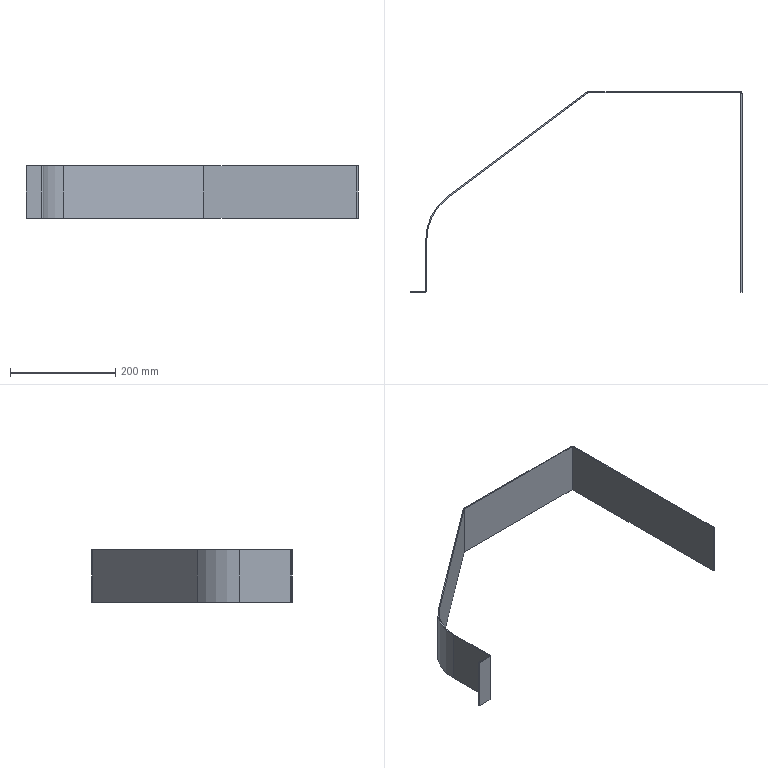Part | SolidWorks | features ICE 5, DeleteBody 4, Split 4, Extrusion 1, FlatPattern 1, SheetMetal 1, Shell 1, SolidToSheetMetal 1 | 1 solid | 38 faces | box 630 x 380 x 100 mm | volume 244808 mm3 | plane 30 | cylinder 8 | commonest cylinder face diameters 2 x3 6 x3 196 x1 200 x1
STEP:
#1=CARTESIAN_POINT('',(-1098.,3.,-198.));
#2=VERTEX_POINT('',#1);
#3=CARTESIAN_POINT('',(-1100.,3.,-198.));
#4=VERTEX_POINT('',#3);
#5=CARTESIAN_POINT('',(-1100.,3.,-198.));
#6=DIRECTION('',(-1.,0.,0.));
#7=VECTOR('',#6,1000.);
#8=LINE('',#5,#7);
#9=EDGE_CURVE('',#2,#4,#8,.T.);
#10=ORIENTED_EDGE('',*,*,#9,.F.);
#11=CARTESIAN_POINT('',(-1098.,100.,-198.));
#12=VERTEX_POINT('',#11);
#13=CARTESIAN_POINT('',(-1098.,100.,-198.));
#14=DIRECTION('',(0.,1.,0.));
#15=VECTOR('',#14,1000.);
#16=LINE('',#13,#15);
#17=EDGE_CURVE('',#2,#12,#16,.T.);
#18=ORIENTED_EDGE('',*,*,#17,.T.);
#19=CARTESIAN_POINT('',(-1100.,100.,-198.));
#20=VERTEX_POINT('',#19);
#21=CARTESIAN_POINT('',(-1100.,100.,-198.));
#22=DIRECTION('',(-1.,0.,0.));
#23=VECTOR('',#22,1000.);
#24=LINE('',#21,#23);
#25=EDGE_CURVE('',#12,#20,#24,.T.);
#26=ORIENTED_EDGE('',*,*,#25,.T.);
#27=CARTESIAN_POINT('',(-1100.,100.,-198.));
#28=DIRECTION('',(0.,1.,0.));
#29=VECTOR('',#28,1000.);
#30=LINE('',#27,#29);
#31=EDGE_CURVE('',#4,#20,#30,.T.);
#32=ORIENTED_EDGE('',*,*,#31,.F.);
#33=EDGE_LOOP('',(#10,#18,#26,#32));
#34=FACE_OUTER_BOUND('',#33,.T.);
#35=CARTESIAN_POINT('',(-1100.,100.,-198.));
#36=DIRECTION('',(0.,0.,1.));
#37=DIRECTION('',(0.,1.,0.));
#38=AXIS2_PLACEMENT_3D('',#35,#36,#37);
#39=PLANE('',#38);
#40=ADVANCED_FACE('',(#34),#39,.T.);
#41=ORIENTED_EDGE('',*,*,#25,.F.);
#42=CARTESIAN_POINT('',(-1058.8,178.4,-198.));
#43=VERTEX_POINT('',#42);
#44=CARTESIAN_POINT('',(-1000.,100.,-198.));
#45=DIRECTION('',(0.,0.,-1.));
#46=DIRECTION('',(1.,0.,0.));
#47=AXIS2_PLACEMENT_3D('',#44,#45,#46);
#48=CIRCLE('',#47,98.);
#49=EDGE_CURVE('',#12,#43,#48,.T.);
#50=ORIENTED_EDGE('',*,*,#49,.T.);
#51=CARTESIAN_POINT('',(-1060.,180.,-198.));
#52=VERTEX_POINT('',#51);
#53=CARTESIAN_POINT('',(-1060.,180.,-198.));
#54=DIRECTION('',(-0.6,0.8,0.));
#55=VECTOR('',#54,1000.);
#56=LINE('',#53,#55);
#57=EDGE_CURVE('',#43,#52,#56,.T.);
#58=ORIENTED_EDGE('',*,*,#57,.T.);
#59=CARTESIAN_POINT('',(-1000.,100.,-198.));
#60=DIRECTION('',(0.,0.,-1.));
#61=DIRECTION('',(1.,0.,0.));
#62=AXIS2_PLACEMENT_3D('',#59,#60,#61);
#63=CIRCLE('',#62,100.);
#64=EDGE_CURVE('',#20,#52,#63,.T.);
#65=ORIENTED_EDGE('',*,*,#64,.F.);
#66=EDGE_LOOP('',(#41,#50,#58,#65));
#67=FACE_OUTER_BOUND('',#66,.T.);
#68=CARTESIAN_POINT('',(-1000.,100.,-198.));
#69=DIRECTION('',(0.,0.,-1.));
#70=DIRECTION('',(-1.,0.,0.));
#71=AXIS2_PLACEMENT_3D('',#68,#69,#70);
#72=PLANE('',#71);
#73=ADVANCED_FACE('',(#67),#72,.F.);
#74=ORIENTED_EDGE('',*,*,#57,.F.);
#75=CARTESIAN_POINT('',(-792.933,377.8,-198.));
#76=VERTEX_POINT('',#75);
#77=CARTESIAN_POINT('',(-1058.8,178.4,-198.));
#78=DIRECTION('',(0.8,0.6,0.));
#79=VECTOR('',#78,1000.);
#80=LINE('',#77,#79);
#81=EDGE_CURVE('',#43,#76,#80,.T.);
#82=ORIENTED_EDGE('',*,*,#81,.T.);
#83=CARTESIAN_POINT('',(-794.133,379.4,-198.));
#84=VERTEX_POINT('',#83);
#85=CARTESIAN_POINT('',(-794.133,379.4,-198.));
#86=DIRECTION('',(-0.6,0.8,0.));
#87=VECTOR('',#86,1000.);
#88=LINE('',#85,#87);
#89=EDGE_CURVE('',#76,#84,#88,.T.);
#90=ORIENTED_EDGE('',*,*,#89,.T.);
#91=CARTESIAN_POINT('',(-1060.,180.,-198.));
#92=DIRECTION('',(0.8,0.6,0.));
#93=VECTOR('',#92,1000.);
#94=LINE('',#91,#93);
#95=EDGE_CURVE('',#52,#84,#94,.T.);
#96=ORIENTED_EDGE('',*,*,#95,.F.);
#97=EDGE_LOOP('',(#74,#82,#90,#96));
#98=FACE_OUTER_BOUND('',#97,.T.);
#99=CARTESIAN_POINT('',(-1060.,180.,-198.));
#100=DIRECTION('',(0.,0.,1.));
#101=DIRECTION('',(0.8,0.6,0.));
#102=AXIS2_PLACEMENT_3D('',#99,#100,#101);
#103=PLANE('',#102);
#104=ADVANCED_FACE('',(#98),#103,.T.);
#105=ORIENTED_EDGE('',*,*,#89,.F.);
#106=CARTESIAN_POINT('',(-792.333,378.,-198.));
#107=VERTEX_POINT('',#106);
#108=CARTESIAN_POINT('',(-792.333,377.,-198.));
#109=DIRECTION('',(0.,0.,-1.));
#110=DIRECTION('',(1.,0.,0.));
#111=AXIS2_PLACEMENT_3D('',#108,#109,#110);
#112=CIRCLE('',#111,1.);
#113=EDGE_CURVE('',#76,#107,#112,.T.);
#114=ORIENTED_EDGE('',*,*,#113,.T.);
#115=CARTESIAN_POINT('',(-792.333,380.,-198.));
#116=VERTEX_POINT('',#115);
#117=CARTESIAN_POINT('',(-792.333,380.,-198.));
#118=DIRECTION('',(0.,1.,0.));
#119=VECTOR('',#118,1000.);
#120=LINE('',#117,#119);
#121=EDGE_CURVE('',#107,#116,#120,.T.);
#122=ORIENTED_EDGE('',*,*,#121,.T.);
#123=CARTESIAN_POINT('',(-792.333,377.,-198.));
#124=DIRECTION('',(0.,0.,-1.));
#125=DIRECTION('',(-1.,0.,0.));
#126=AXIS2_PLACEMENT_3D('',#123,#124,#125);
#127=CIRCLE('',#126,3.);
#128=EDGE_CURVE('',#84,#116,#127,.T.);
#129=ORIENTED_EDGE('',*,*,#128,.F.);
#130=EDGE_LOOP('',(#105,#114,#122,#129));
#131=FACE_OUTER_BOUND('',#130,.T.);
#132=CARTESIAN_POINT('',(-792.333,377.,-198.));
#133=DIRECTION('',(0.,0.,1.));
#134=DIRECTION('',(1.,0.,0.));
#135=AXIS2_PLACEMENT_3D('',#132,#133,#134);
#136=PLANE('',#135);
#137=ADVANCED_FACE('',(#131),#136,.T.);
#138=ORIENTED_EDGE('',*,*,#121,.F.);
#139=CARTESIAN_POINT('',(-503.,378.,-198.));
#140=VERTEX_POINT('',#139);
#141=CARTESIAN_POINT('',(-500.,378.,-198.));
#142=DIRECTION('',(-1.,0.,0.));
#143=VECTOR('',#142,1000.);
#144=LINE('',#141,#143);
#145=EDGE_CURVE('',#140,#107,#144,.T.);
#146=ORIENTED_EDGE('',*,*,#145,.F.);
#147=CARTESIAN_POINT('',(-503.,380.,-198.));
#148=VERTEX_POINT('',#147);
#149=CARTESIAN_POINT('',(-503.,380.,-198.));
#150=DIRECTION('',(0.,1.,0.));
#151=VECTOR('',#150,1000.);
#152=LINE('',#149,#151);
#153=EDGE_CURVE('',#140,#148,#152,.T.);
#154=ORIENTED_EDGE('',*,*,#153,.T.);
#155=CARTESIAN_POINT('',(-2.,380.,-198.));
#156=DIRECTION('',(-1.,0.,0.));
#157=VECTOR('',#156,1000.);
#158=LINE('',#155,#157);
#159=EDGE_CURVE('',#148,#116,#158,.T.);
#160=ORIENTED_EDGE('',*,*,#159,.T.);
#161=EDGE_LOOP('',(#138,#146,#154,#160));
#162=FACE_OUTER_BOUND('',#161,.T.);
#163=CARTESIAN_POINT('',(-2.,380.,-198.));
#164=DIRECTION('',(0.,0.,-1.));
#165=DIRECTION('',(-1.,0.,0.));
#166=AXIS2_PLACEMENT_3D('',#163,#164,#165);
#167=PLANE('',#166);
#168=ADVANCED_FACE('',(#162),#167,.F.);
#169=ORIENTED_EDGE('',*,*,#153,.F.);
#170=CARTESIAN_POINT('',(-502.,377.,-198.));
#171=VERTEX_POINT('',#170);
#172=CARTESIAN_POINT('',(-503.,377.,-198.));
#173=DIRECTION('',(0.,0.,-1.));
#174=DIRECTION('',(1.,0.,0.));
#175=AXIS2_PLACEMENT_3D('',#172,#173,#174);
#176=CIRCLE('',#175,1.);
#177=EDGE_CURVE('',#140,#171,#176,.T.);
#178=ORIENTED_EDGE('',*,*,#177,.T.);
#179=CARTESIAN_POINT('',(-500.,377.,-198.));
#180=VERTEX_POINT('',#179);
#181=CARTESIAN_POINT('',(-500.,377.,-198.));
#182=DIRECTION('',(1.,0.,0.));
#183=VECTOR('',#182,1000.);
#184=LINE('',#181,#183);
#185=EDGE_CURVE('',#171,#180,#184,.T.);
#186=ORIENTED_EDGE('',*,*,#185,.T.);
#187=CARTESIAN_POINT('',(-503.,377.,-198.));
#188=DIRECTION('',(0.,0.,-1.));
#189=DIRECTION('',(1.,0.,0.));
#190=AXIS2_PLACEMENT_3D('',#187,#188,#189);
#191=CIRCLE('',#190,3.);
#192=EDGE_CURVE('',#148,#180,#191,.T.);
#193=ORIENTED_EDGE('',*,*,#192,.F.);
#194=EDGE_LOOP('',(#169,#178,#186,#193));
#195=FACE_OUTER_BOUND('',#194,.T.);
#196=CARTESIAN_POINT('',(-503.,377.,-198.));
#197=DIRECTION('',(0.,0.,-1.));
#198=DIRECTION('',(-1.,0.,0.));
#199=AXIS2_PLACEMENT_3D('',#196,#197,#198);
#200=PLANE('',#199);
#201=ADVANCED_FACE('',(#195),#200,.F.);
#202=ORIENTED_EDGE('',*,*,#185,.F.);
#203=CARTESIAN_POINT('',(-502.,0.,-198.));
#204=VERTEX_POINT('',#203);
#205=CARTESIAN_POINT('',(-502.,2.,-198.));
#206=DIRECTION('',(0.,1.,0.));
#207=VECTOR('',#206,1000.);
#208=LINE('',#205,#207);
#209=EDGE_CURVE('',#204,#171,#208,.T.);
#210=ORIENTED_EDGE('',*,*,#209,.F.);
#211=CARTESIAN_POINT('',(-500.,0.,-198.));
#212=VERTEX_POINT('',#211);
#213=CARTESIAN_POINT('',(-500.,0.,-198.));
#214=DIRECTION('',(1.,0.,0.));
#215=VECTOR('',#214,1000.);
#216=LINE('',#213,#215);
#217=EDGE_CURVE('',#204,#212,#216,.T.);
#218=ORIENTED_EDGE('',*,*,#217,.T.);
#219=CARTESIAN_POINT('',(-500.,375.,-198.));
#220=DIRECTION('',(0.,1.,0.));
#221=VECTOR('',#220,1000.);
#222=LINE('',#219,#221);
#223=EDGE_CURVE('',#212,#180,#222,.T.);
#224=ORIENTED_EDGE('',*,*,#223,.T.);
#225=EDGE_LOOP('',(#202,#210,#218,#224));
#226=FACE_OUTER_BOUND('',#225,.T.);
#227=CARTESIAN_POINT('',(-500.,375.,-198.));
#228=DIRECTION('',(0.,0.,-1.));
#229=DIRECTION('',(0.,1.,0.));
#230=AXIS2_PLACEMENT_3D('',#227,#228,#229);
#231=PLANE('',#230);
#232=ADVANCED_FACE('',(#226),#231,.F.);
#233=ORIENTED_EDGE('',*,*,#217,.F.);
#234=CARTESIAN_POINT('',(-502.,0.,-298.));
#235=VERTEX_POINT('',#234);
#236=CARTESIAN_POINT('',(-502.,0.,-200.));
#237=DIRECTION('',(0.,0.,1.));
#238=VECTOR('',#237,1000.);
#239=LINE('',#236,#238);
#240=EDGE_CURVE('',#235,#204,#239,.T.);
#241=ORIENTED_EDGE('',*,*,#240,.F.);
#242=CARTESIAN_POINT('',(-500.,0.,-298.));
#243=VERTEX_POINT('',#242);
#244=CARTESIAN_POINT('',(-500.,0.,-298.));
#245=DIRECTION('',(1.,0.,0.));
#246=VECTOR('',#245,1000.);
#247=LINE('',#244,#246);
#248=EDGE_CURVE('',#235,#243,#247,.T.);
#249=ORIENTED_EDGE('',*,*,#248,.T.);
#250=CARTESIAN_POINT('',(-500.,0.,-200.));
#251=DIRECTION('',(0.,0.,1.));
#252=VECTOR('',#251,1000.);
#253=LINE('',#250,#252);
#254=EDGE_CURVE('',#243,#212,#253,.T.);
#255=ORIENTED_EDGE('',*,*,#254,.T.);
#256=EDGE_LOOP('',(#233,#241,#249,#255));
#257=FACE_OUTER_BOUND('',#256,.T.);
#258=CARTESIAN_POINT('',(-500.,0.,-200.));
#259=DIRECTION('',(0.,1.,0.));
#260=DIRECTION('',(0.,0.,1.));
#261=AXIS2_PLACEMENT_3D('',#258,#259,#260);
#262=PLANE('',#261);
#263=ADVANCED_FACE('',(#257),#262,.F.);
#264=ORIENTED_EDGE('',*,*,#248,.F.);
#265=CARTESIAN_POINT('',(-502.,377.,-298.));
#266=VERTEX_POINT('',#265);
#267=CARTESIAN_POINT('',(-502.,2.,-298.));
#268=DIRECTION('',(0.,-1.,0.));
#269=VECTOR('',#268,1000.);
#270=LINE('',#267,#269);
#271=EDGE_CURVE('',#266,#235,#270,.T.);
#272=ORIENTED_EDGE('',*,*,#271,.F.);
#273=CARTESIAN_POINT('',(-500.,377.,-298.));
#274=VERTEX_POINT('',#273);
#275=CARTESIAN_POINT('',(-500.,377.,-298.));
#276=DIRECTION('',(1.,0.,0.));
#277=VECTOR('',#276,1000.);
#278=LINE('',#275,#277);
#279=EDGE_CURVE('',#266,#274,#278,.T.);
#280=ORIENTED_EDGE('',*,*,#279,.T.);
#281=CARTESIAN_POINT('',(-500.,2.,-298.));
#282=DIRECTION('',(0.,-1.,0.));
#283=VECTOR('',#282,1000.);
#284=LINE('',#281,#283);
#285=EDGE_CURVE('',#274,#243,#284,.T.);
#286=ORIENTED_EDGE('',*,*,#285,.T.);
#287=EDGE_LOOP('',(#264,#272,#280,#286));
#288=FACE_OUTER_BOUND('',#287,.T.);
#289=CARTESIAN_POINT('',(-500.,2.,-298.));
#290=DIRECTION('',(0.,0.,1.));
#291=DIRECTION('',(0.,-1.,0.));
#292=AXIS2_PLACEMENT_3D('',#289,#290,#291);
#293=PLANE('',#292);
#294=ADVANCED_FACE('',(#288),#293,.F.);
#295=ORIENTED_EDGE('',*,*,#279,.F.);
#296=CARTESIAN_POINT('',(-503.,378.,-298.));
#297=VERTEX_POINT('',#296);
#298=CARTESIAN_POINT('',(-503.,377.,-298.));
#299=DIRECTION('',(0.,0.,1.));
#300=DIRECTION('',(1.,0.,0.));
#301=AXIS2_PLACEMENT_3D('',#298,#299,#300);
#302=CIRCLE('',#301,1.);
#303=EDGE_CURVE('',#266,#297,#302,.T.);
#304=ORIENTED_EDGE('',*,*,#303,.T.);
#305=CARTESIAN_POINT('',(-503.,380.,-298.));
#306=VERTEX_POINT('',#305);
#307=CARTESIAN_POINT('',(-503.,380.,-298.));
#308=DIRECTION('',(0.,1.,0.));
#309=VECTOR('',#308,1000.);
#310=LINE('',#307,#309);
#311=EDGE_CURVE('',#297,#306,#310,.T.);
#312=ORIENTED_EDGE('',*,*,#311,.T.);
#313=CARTESIAN_POINT('',(-503.,377.,-298.));
#314=DIRECTION('',(0.,0.,1.));
#315=DIRECTION('',(-1.,0.,0.));
#316=AXIS2_PLACEMENT_3D('',#313,#314,#315);
#317=CIRCLE('',#316,3.);
#318=EDGE_CURVE('',#274,#306,#317,.T.);
#319=ORIENTED_EDGE('',*,*,#318,.F.);
#320=EDGE_LOOP('',(#295,#304,#312,#319));
#321=FACE_OUTER_BOUND('',#320,.T.);
#322=CARTESIAN_POINT('',(-503.,377.,-298.));
#323=DIRECTION('',(0.,0.,1.));
#324=DIRECTION('',(1.,0.,0.));
#325=AXIS2_PLACEMENT_3D('',#322,#323,#324);
#326=PLANE('',#325);
#327=ADVANCED_FACE('',(#321),#326,.F.);
#328=ORIENTED_EDGE('',*,*,#311,.F.);
#329=CARTESIAN_POINT('',(-792.333,378.,-298.));
#330=VERTEX_POINT('',#329);
#331=CARTESIAN_POINT('',(-500.,378.,-298.));
#332=DIRECTION('',(1.,0.,0.));
#333=VECTOR('',#332,1000.);
#334=LINE('',#331,#333);
#335=EDGE_CURVE('',#330,#297,#334,.T.);
#336=ORIENTED_EDGE('',*,*,#335,.F.);
#337=CARTESIAN_POINT('',(-792.333,380.,-298.));
#338=VERTEX_POINT('',#337);
#339=CARTESIAN_POINT('',(-792.333,380.,-298.));
#340=DIRECTION('',(0.,1.,0.));
#341=VECTOR('',#340,1000.);
#342=LINE('',#339,#341);
#343=EDGE_CURVE('',#330,#338,#342,.T.);
#344=ORIENTED_EDGE('',*,*,#343,.T.);
#345=CARTESIAN_POINT('',(-500.,380.,-298.));
#346=DIRECTION('',(1.,0.,0.));
#347=VECTOR('',#346,1000.);
#348=LINE('',#345,#347);
#349=EDGE_CURVE('',#338,#306,#348,.T.);
#350=ORIENTED_EDGE('',*,*,#349,.T.);
#351=EDGE_LOOP('',(#328,#336,#344,#350));
#352=FACE_OUTER_BOUND('',#351,.T.);
#353=CARTESIAN_POINT('',(-500.,380.,-298.));
#354=DIRECTION('',(0.,0.,1.));
#355=DIRECTION('',(1.,0.,0.));
#356=AXIS2_PLACEMENT_3D('',#353,#354,#355);
#357=PLANE('',#356);
#358=ADVANCED_FACE('',(#352),#357,.F.);
#359=ORIENTED_EDGE('',*,*,#343,.F.);
#360=CARTESIAN_POINT('',(-792.933,377.8,-298.));
#361=VERTEX_POINT('',#360);
#362=CARTESIAN_POINT('',(-792.333,377.,-298.));
#363=DIRECTION('',(0.,0.,1.));
#364=DIRECTION('',(1.,0.,0.));
#365=AXIS2_PLACEMENT_3D('',#362,#363,#364);
#366=CIRCLE('',#365,1.);
#367=EDGE_CURVE('',#330,#361,#366,.T.);
#368=ORIENTED_EDGE('',*,*,#367,.T.);
#369=CARTESIAN_POINT('',(-794.133,379.4,-298.));
#370=VERTEX_POINT('',#369);
#371=CARTESIAN_POINT('',(-794.133,379.4,-298.));
#372=DIRECTION('',(-0.6,0.8,0.));
#373=VECTOR('',#372,1000.);
#374=LINE('',#371,#373);
#375=EDGE_CURVE('',#361,#370,#374,.T.);
#376=ORIENTED_EDGE('',*,*,#375,.T.);
#377=CARTESIAN_POINT('',(-792.333,377.,-298.));
#378=DIRECTION('',(0.,0.,1.));
#379=DIRECTION('',(-1.,0.,0.));
#380=AXIS2_PLACEMENT_3D('',#377,#378,#379);
#381=CIRCLE('',#380,3.);
#382=EDGE_CURVE('',#338,#370,#381,.T.);
#383=ORIENTED_EDGE('',*,*,#382,.F.);
#384=EDGE_LOOP('',(#359,#368,#376,#383));
#385=FACE_OUTER_BOUND('',#384,.T.);
#386=CARTESIAN_POINT('',(-792.333,377.,-298.));
#387=DIRECTION('',(0.,0.,1.));
#388=DIRECTION('',(1.,0.,0.));
#389=AXIS2_PLACEMENT_3D('',#386,#387,#388);
#390=PLANE('',#389);
#391=ADVANCED_FACE('',(#385),#390,.F.);
#392=ORIENTED_EDGE('',*,*,#375,.F.);
#393=CARTESIAN_POINT('',(-1058.8,178.4,-298.));
#394=VERTEX_POINT('',#393);
#395=CARTESIAN_POINT('',(-1058.8,178.4,-298.));
#396=DIRECTION('',(0.8,0.6,0.));
#397=VECTOR('',#396,1000.);
#398=LINE('',#395,#397);
#399=EDGE_CURVE('',#394,#361,#398,.T.);
#400=ORIENTED_EDGE('',*,*,#399,.F.);
#401=CARTESIAN_POINT('',(-1060.,180.,-298.));
#402=VERTEX_POINT('',#401);
#403=CARTESIAN_POINT('',(-1060.,180.,-298.));
#404=DIRECTION('',(-0.6,0.8,0.));
#405=VECTOR('',#404,1000.);
#406=LINE('',#403,#405);
#407=EDGE_CURVE('',#394,#402,#406,.T.);
#408=ORIENTED_EDGE('',*,*,#407,.T.);
#409=CARTESIAN_POINT('',(-1060.,180.,-298.));
#410=DIRECTION('',(0.8,0.6,0.));
#411=VECTOR('',#410,1000.);
#412=LINE('',#409,#411);
#413=EDGE_CURVE('',#402,#370,#412,.T.);
#414=ORIENTED_EDGE('',*,*,#413,.T.);
#415=EDGE_LOOP('',(#392,#400,#408,#414));
#416=FACE_OUTER_BOUND('',#415,.T.);
#417=CARTESIAN_POINT('',(-1060.,180.,-298.));
#418=DIRECTION('',(0.,0.,1.));
#419=DIRECTION('',(0.8,0.6,0.));
#420=AXIS2_PLACEMENT_3D('',#417,#418,#419);
#421=PLANE('',#420);
#422=ADVANCED_FACE('',(#416),#421,.F.);
#423=ORIENTED_EDGE('',*,*,#407,.F.);
#424=CARTESIAN_POINT('',(-1098.,100.,-298.));
#425=VERTEX_POINT('',#424);
#426=CARTESIAN_POINT('',(-1000.,100.,-298.));
#427=DIRECTION('',(0.,0.,-1.));
#428=DIRECTION('',(1.,0.,0.));
#429=AXIS2_PLACEMENT_3D('',#426,#427,#428);
#430=CIRCLE('',#429,98.);
#431=EDGE_CURVE('',#425,#394,#430,.T.);
#432=ORIENTED_EDGE('',*,*,#431,.F.);
#433=CARTESIAN_POINT('',(-1100.,100.,-298.));
#434=VERTEX_POINT('',#433);
#435=CARTESIAN_POINT('',(-1100.,100.,-298.));
#436=DIRECTION('',(-1.,0.,0.));
#437=VECTOR('',#436,1000.);
#438=LINE('',#435,#437);
#439=EDGE_CURVE('',#425,#434,#438,.T.);
#440=ORIENTED_EDGE('',*,*,#439,.T.);
#441=CARTESIAN_POINT('',(-1000.,100.,-298.));
#442=DIRECTION('',(0.,0.,-1.));
#443=DIRECTION('',(1.,0.,0.));
#444=AXIS2_PLACEMENT_3D('',#441,#442,#443);
#445=CIRCLE('',#444,100.);
#446=EDGE_CURVE('',#434,#402,#445,.T.);
#447=ORIENTED_EDGE('',*,*,#446,.T.);
#448=EDGE_LOOP('',(#423,#432,#440,#447));
#449=FACE_OUTER_BOUND('',#448,.T.);
#450=CARTESIAN_POINT('',(-1000.,100.,-298.));
#451=DIRECTION('',(0.,0.,-1.));
#452=DIRECTION('',(-1.,0.,0.));
#453=AXIS2_PLACEMENT_3D('',#450,#451,#452);
#454=PLANE('',#453);
#455=ADVANCED_FACE('',(#449),#454,.T.);
#456=ORIENTED_EDGE('',*,*,#439,.F.);
#457=CARTESIAN_POINT('',(-1098.,3.,-298.));
#458=VERTEX_POINT('',#457);
#459=CARTESIAN_POINT('',(-1098.,100.,-298.));
#460=DIRECTION('',(0.,1.,0.));
#461=VECTOR('',#460,1000.);
#462=LINE('',#459,#461);
#463=EDGE_CURVE('',#458,#425,#462,.T.);
#464=ORIENTED_EDGE('',*,*,#463,.F.);
#465=CARTESIAN_POINT('',(-1100.,3.,-298.));
#466=VERTEX_POINT('',#465);
#467=CARTESIAN_POINT('',(-1100.,3.,-298.));
#468=DIRECTION('',(-1.,0.,0.));
#469=VECTOR('',#468,1000.);
#470=LINE('',#467,#469);
#471=EDGE_CURVE('',#458,#466,#470,.T.);
#472=ORIENTED_EDGE('',*,*,#471,.T.);
#473=CARTESIAN_POINT('',(-1100.,100.,-298.));
#474=DIRECTION('',(0.,1.,0.));
#475=VECTOR('',#474,1000.);
#476=LINE('',#473,#475);
#477=EDGE_CURVE('',#466,#434,#476,.T.);
#478=ORIENTED_EDGE('',*,*,#477,.T.);
#479=EDGE_LOOP('',(#456,#464,#472,#478));
#480=FACE_OUTER_BOUND('',#479,.T.);
#481=CARTESIAN_POINT('',(-1100.,100.,-298.));
#482=DIRECTION('',(0.,0.,1.));
#483=DIRECTION('',(0.,1.,0.));
#484=AXIS2_PLACEMENT_3D('',#481,#482,#483);
#485=PLANE('',#484);
#486=ADVANCED_FACE('',(#480),#485,.F.);
#487=ORIENTED_EDGE('',*,*,#471,.F.);
#488=CARTESIAN_POINT('',(-1101.,0.,-298.));
#489=VERTEX_POINT('',#488);
#490=CARTESIAN_POINT('',(-1101.,3.,-298.));
#491=DIRECTION('',(0.,0.,-1.));
#492=DIRECTION('',(-1.,0.,0.));
#493=AXIS2_PLACEMENT_3D('',#490,#491,#492);
#494=CIRCLE('',#493,3.);
#495=EDGE_CURVE('',#458,#489,#494,.T.);
#496=ORIENTED_EDGE('',*,*,#495,.T.);
#497=CARTESIAN_POINT('',(-1101.,2.,-298.));
#498=VERTEX_POINT('',#497);
#499=CARTESIAN_POINT('',(-1101.,2.,-298.));
#500=DIRECTION('',(0.,1.,0.));
#501=VECTOR('',#500,1000.);
#502=LINE('',#499,#501);
#503=EDGE_CURVE('',#489,#498,#502,.T.);
#504=ORIENTED_EDGE('',*,*,#503,.T.);
#505=CARTESIAN_POINT('',(-1101.,3.,-298.));
#506=DIRECTION('',(0.,0.,-1.));
#507=DIRECTION('',(1.,0.,0.));
#508=AXIS2_PLACEMENT_3D('',#505,#506,#507);
#509=CIRCLE('',#508,1.);
#510=EDGE_CURVE('',#466,#498,#509,.T.);
#511=ORIENTED_EDGE('',*,*,#510,.F.);
#512=EDGE_LOOP('',(#487,#496,#504,#511));
#513=FACE_OUTER_BOUND('',#512,.T.);
#514=CARTESIAN_POINT('',(-1101.,3.,-298.));
#515=DIRECTION('',(0.,0.,-1.));
#516=DIRECTION('',(-1.,0.,0.));
#517=AXIS2_PLACEMENT_3D('',#514,#515,#516);
#518=PLANE('',#517);
#519=ADVANCED_FACE('',(#513),#518,.T.);
#520=ORIENTED_EDGE('',*,*,#503,.F.);
#521=CARTESIAN_POINT('',(-1130.,0.,-298.));
#522=VERTEX_POINT('',#521);
#523=CARTESIAN_POINT('',(0.,0.,-298.));
#524=DIRECTION('',(1.,0.,0.));
#525=VECTOR('',#524,1000.);
#526=LINE('',#523,#525);
#527=EDGE_CURVE('',#522,#489,#526,.T.);
#528=ORIENTED_EDGE('',*,*,#527,.F.);
#529=CARTESIAN_POINT('',(-1130.,2.,-298.));
#530=VERTEX_POINT('',#529);
#531=CARTESIAN_POINT('',(-1130.,2.,-298.));
#532=DIRECTION('',(0.,1.,0.));
#533=VECTOR('',#532,1000.);
#534=LINE('',#531,#533);
#535=EDGE_CURVE('',#522,#530,#534,.T.);
#536=ORIENTED_EDGE('',*,*,#535,.T.);
#537=CARTESIAN_POINT('',(0.,2.,-298.));
#538=DIRECTION('',(1.,0.,0.));
#539=VECTOR('',#538,1000.);
#540=LINE('',#537,#539);
#541=EDGE_CURVE('',#530,#498,#540,.T.);
#542=ORIENTED_EDGE('',*,*,#541,.T.);
#543=EDGE_LOOP('',(#520,#528,#536,#542));
#544=FACE_OUTER_BOUND('',#543,.T.);
#545=CARTESIAN_POINT('',(0.,2.,-298.));
#546=DIRECTION('',(0.,0.,1.));
#547=DIRECTION('',(1.,0.,0.));
#548=AXIS2_PLACEMENT_3D('',#545,#546,#547);
#549=PLANE('',#548);
#550=ADVANCED_FACE('',(#544),#549,.F.);
#551=ORIENTED_EDGE('',*,*,#535,.F.);
#552=CARTESIAN_POINT('',(-1130.,0.,-198.));
#553=VERTEX_POINT('',#552);
#554=CARTESIAN_POINT('',(-1130.,0.,0.));
#555=DIRECTION('',(0.,0.,-1.));
#556=VECTOR('',#555,1000.);
#557=LINE('',#554,#556);
#558=EDGE_CURVE('',#553,#522,#557,.T.);
#559=ORIENTED_EDGE('',*,*,#558,.F.);
#560=CARTESIAN_POINT('',(-1130.,2.,-198.));
#561=VERTEX_POINT('',#560);
#562=CARTESIAN_POINT('',(-1130.,2.,-198.));
#563=DIRECTION('',(0.,1.,0.));
#564=VECTOR('',#563,1000.);
#565=LINE('',#562,#564);
#566=EDGE_CURVE('',#553,#561,#565,.T.);
#567=ORIENTED_EDGE('',*,*,#566,.T.);
#568=CARTESIAN_POINT('',(-1130.,2.,0.));
#569=DIRECTION('',(0.,0.,-1.));
#570=VECTOR('',#569,1000.);
#571=LINE('',#568,#570);
#572=EDGE_CURVE('',#561,#530,#571,.T.);
#573=ORIENTED_EDGE('',*,*,#572,.T.);
#574=EDGE_LOOP('',(#551,#559,#567,#573));
#575=FACE_OUTER_BOUND('',#574,.T.);
#576=CARTESIAN_POINT('',(-1130.,2.,0.));
#577=DIRECTION('',(1.,0.,0.));
#578=DIRECTION('',(0.,0.,-1.));
#579=AXIS2_PLACEMENT_3D('',#576,#577,#578);
#580=PLANE('',#579);
#581=ADVANCED_FACE('',(#575),#580,.F.);
#582=ORIENTED_EDGE('',*,*,#566,.F.);
#583=CARTESIAN_POINT('',(-1101.,0.,-198.));
#584=VERTEX_POINT('',#583);
#585=CARTESIAN_POINT('',(0.,0.,-198.));
#586=DIRECTION('',(1.,0.,0.));
#587=VECTOR('',#586,1000.);
#588=LINE('',#585,#587);
#589=EDGE_CURVE('',#553,#584,#588,.T.);
#590=ORIENTED_EDGE('',*,*,#589,.T.);
#591=CARTESIAN_POINT('',(-1101.,2.,-198.));
#592=VERTEX_POINT('',#591);
#593=CARTESIAN_POINT('',(-1101.,2.,-198.));
#594=DIRECTION('',(0.,1.,0.));
#595=VECTOR('',#594,1000.);
#596=LINE('',#593,#595);
#597=EDGE_CURVE('',#584,#592,#596,.T.);
#598=ORIENTED_EDGE('',*,*,#597,.T.);
#599=CARTESIAN_POINT('',(0.,2.,-198.));
#600=DIRECTION('',(1.,0.,0.));
#601=VECTOR('',#600,1000.);
#602=LINE('',#599,#601);
#603=EDGE_CURVE('',#561,#592,#602,.T.);
#604=ORIENTED_EDGE('',*,*,#603,.F.);
#605=EDGE_LOOP('',(#582,#590,#598,#604));
#606=FACE_OUTER_BOUND('',#605,.T.);
#607=CARTESIAN_POINT('',(0.,2.,-198.));
#608=DIRECTION('',(0.,0.,1.));
#609=DIRECTION('',(1.,0.,0.));
#610=AXIS2_PLACEMENT_3D('',#607,#608,#609);
#611=PLANE('',#610);
#612=ADVANCED_FACE('',(#606),#611,.T.);
#613=CARTESIAN_POINT('',(-1101.,3.,-198.));
#614=DIRECTION('',(0.,0.,1.));
#615=DIRECTION('',(-1.,0.,0.));
#616=AXIS2_PLACEMENT_3D('',#613,#614,#615);
#617=CIRCLE('',#616,3.);
#618=EDGE_CURVE('',#584,#2,#617,.T.);
#619=ORIENTED_EDGE('',*,*,#618,.T.);
#620=ORIENTED_EDGE('',*,*,#9,.T.);
#621=CARTESIAN_POINT('',(-1101.,3.,-198.));
#622=DIRECTION('',(0.,0.,1.));
#623=DIRECTION('',(-1.,0.,0.));
#624=AXIS2_PLACEMENT_3D('',#621,#622,#623);
#625=CIRCLE('',#624,1.);
#626=EDGE_CURVE('',#592,#4,#625,.T.);
#627=ORIENTED_EDGE('',*,*,#626,.F.);
#628=ORIENTED_EDGE('',*,*,#597,.F.);
#629=EDGE_LOOP('',(#619,#620,#627,#628));
#630=FACE_OUTER_BOUND('',#629,.T.);
#631=CARTESIAN_POINT('',(-1101.,3.,-198.));
#632=DIRECTION('',(0.,0.,1.));
#633=DIRECTION('',(1.,0.,0.));
#634=AXIS2_PLACEMENT_3D('',#631,#632,#633);
#635=PLANE('',#634);
#636=ADVANCED_FACE('',(#630),#635,.T.);
#637=ORIENTED_EDGE('',*,*,#603,.T.);
#638=CARTESIAN_POINT('',(-1101.,2.,-298.));
#639=DIRECTION('',(0.,0.,-1.));
#640=VECTOR('',#639,1000.);
#641=LINE('',#638,#640);
#642=EDGE_CURVE('',#592,#498,#641,.T.);
#643=ORIENTED_EDGE('',*,*,#642,.T.);
#644=ORIENTED_EDGE('',*,*,#541,.F.);
#645=ORIENTED_EDGE('',*,*,#572,.F.);
#646=EDGE_LOOP('',(#637,#643,#644,#645));
#647=FACE_OUTER_BOUND('',#646,.T.);
#648=CARTESIAN_POINT('',(0.,2.,0.));
#649=DIRECTION('',(0.,1.,0.));
#650=DIRECTION('',(0.,0.,1.));
#651=AXIS2_PLACEMENT_3D('',#648,#649,#650);
#652=PLANE('',#651);
#653=ADVANCED_FACE('',(#647),#652,.T.);
#654=ORIENTED_EDGE('',*,*,#446,.F.);
#655=CARTESIAN_POINT('',(-1100.,100.,-200.));
#656=DIRECTION('',(0.,0.,1.));
#657=VECTOR('',#656,1000.);
#658=LINE('',#655,#657);
#659=EDGE_CURVE('',#434,#20,#658,.T.);
#660=ORIENTED_EDGE('',*,*,#659,.T.);
#661=ORIENTED_EDGE('',*,*,#64,.T.);
#662=CARTESIAN_POINT('',(-1060.,180.,-200.));
#663=DIRECTION('',(0.,0.,1.));
#664=VECTOR('',#663,1000.);
#665=LINE('',#662,#664);
#666=EDGE_CURVE('',#402,#52,#665,.T.);
#667=ORIENTED_EDGE('',*,*,#666,.F.);
#668=EDGE_LOOP('',(#654,#660,#661,#667));
#669=FACE_OUTER_BOUND('',#668,.T.);
#670=CARTESIAN_POINT('',(-1000.,100.,-200.));
#671=DIRECTION('',(0.,0.,1.));
#672=DIRECTION('',(1.,0.,0.));
#673=AXIS2_PLACEMENT_3D('',#670,#671,#672);
#674=CYLINDRICAL_SURFACE('',#673,100.);
#675=ADVANCED_FACE('',(#669),#674,.T.);
#676=ORIENTED_EDGE('',*,*,#477,.F.);
#677=CARTESIAN_POINT('',(-1100.,3.,-198.));
#678=DIRECTION('',(0.,0.,1.));
#679=VECTOR('',#678,1000.);
#680=LINE('',#677,#679);
#681=EDGE_CURVE('',#466,#4,#680,.T.);
#682=ORIENTED_EDGE('',*,*,#681,.T.);
#683=ORIENTED_EDGE('',*,*,#31,.T.);
#684=ORIENTED_EDGE('',*,*,#659,.F.);
#685=EDGE_LOOP('',(#676,#682,#683,#684));
#686=FACE_OUTER_BOUND('',#685,.T.);
#687=CARTESIAN_POINT('',(-1100.,100.,-200.));
#688=DIRECTION('',(-1.,0.,0.));
#689=DIRECTION('',(0.,0.,1.));
#690=AXIS2_PLACEMENT_3D('',#687,#688,#689);
#691=PLANE('',#690);
#692=ADVANCED_FACE('',(#686),#691,.T.);
#693=ORIENTED_EDGE('',*,*,#95,.T.);
#694=CARTESIAN_POINT('',(-794.133,379.4,-200.));
#695=DIRECTION('',(0.,0.,-1.));
#696=VECTOR('',#695,1000.);
#697=LINE('',#694,#696);
#698=EDGE_CURVE('',#84,#370,#697,.T.);
#699=ORIENTED_EDGE('',*,*,#698,.T.);
#700=ORIENTED_EDGE('',*,*,#413,.F.);
#701=ORIENTED_EDGE('',*,*,#666,.T.);
#702=EDGE_LOOP('',(#693,#699,#700,#701));
#703=FACE_OUTER_BOUND('',#702,.T.);
#704=CARTESIAN_POINT('',(-1060.,180.,-200.));
#705=DIRECTION('',(-0.6,0.8,0.));
#706=DIRECTION('',(-0.8,-0.6,0.));
#707=AXIS2_PLACEMENT_3D('',#704,#705,#706);
#708=PLANE('',#707);
#709=ADVANCED_FACE('',(#703),#708,.T.);
#710=ORIENTED_EDGE('',*,*,#159,.F.);
#711=CARTESIAN_POINT('',(-503.,380.,-200.));
#712=DIRECTION('',(0.,0.,-1.));
#713=VECTOR('',#712,1000.);
#714=LINE('',#711,#713);
#715=EDGE_CURVE('',#148,#306,#714,.T.);
#716=ORIENTED_EDGE('',*,*,#715,.T.);
#717=ORIENTED_EDGE('',*,*,#349,.F.);
#718=CARTESIAN_POINT('',(-792.333,380.,-200.));
#719=DIRECTION('',(0.,0.,1.));
#720=VECTOR('',#719,1000.);
#721=LINE('',#718,#720);
#722=EDGE_CURVE('',#338,#116,#721,.T.);
#723=ORIENTED_EDGE('',*,*,#722,.T.);
#724=EDGE_LOOP('',(#710,#716,#717,#723));
#725=FACE_OUTER_BOUND('',#724,.T.);
#726=CARTESIAN_POINT('',(-500.,380.,-200.));
#727=DIRECTION('',(0.,1.,0.));
#728=DIRECTION('',(-1.,0.,0.));
#729=AXIS2_PLACEMENT_3D('',#726,#727,#728);
#730=PLANE('',#729);
#731=ADVANCED_FACE('',(#725),#730,.T.);
#732=ORIENTED_EDGE('',*,*,#285,.F.);
#733=CARTESIAN_POINT('',(-500.,377.,-200.));
#734=DIRECTION('',(0.,0.,1.));
#735=VECTOR('',#734,1000.);
#736=LINE('',#733,#735);
#737=EDGE_CURVE('',#274,#180,#736,.T.);
#738=ORIENTED_EDGE('',*,*,#737,.T.);
#739=ORIENTED_EDGE('',*,*,#223,.F.);
#740=ORIENTED_EDGE('',*,*,#254,.F.);
#741=EDGE_LOOP('',(#732,#738,#739,#740));
#742=FACE_OUTER_BOUND('',#741,.T.);
#743=CARTESIAN_POINT('',(-500.,2.,-200.));
#744=DIRECTION('',(1.,0.,0.));
#745=DIRECTION('',(0.,0.,-1.));
#746=AXIS2_PLACEMENT_3D('',#743,#744,#745);
#747=PLANE('',#746);
#748=ADVANCED_FACE('',(#742),#747,.T.);
#749=ORIENTED_EDGE('',*,*,#510,.T.);
#750=ORIENTED_EDGE('',*,*,#642,.F.);
#751=ORIENTED_EDGE('',*,*,#626,.T.);
#752=ORIENTED_EDGE('',*,*,#681,.F.);
#753=EDGE_LOOP('',(#749,#750,#751,#752));
#754=FACE_OUTER_BOUND('',#753,.T.);
#755=CARTESIAN_POINT('',(-1101.,3.,-200.));
#756=DIRECTION('',(0.,0.,-1.));
#757=DIRECTION('',(-1.,0.,0.));
#758=AXIS2_PLACEMENT_3D('',#755,#756,#757);
#759=CYLINDRICAL_SURFACE('',#758,1.);
#760=ADVANCED_FACE('',(#754),#759,.F.);
#761=ORIENTED_EDGE('',*,*,#382,.T.);
#762=ORIENTED_EDGE('',*,*,#698,.F.);
#763=ORIENTED_EDGE('',*,*,#128,.T.);
#764=ORIENTED_EDGE('',*,*,#722,.F.);
#765=EDGE_LOOP('',(#761,#762,#763,#764));
#766=FACE_OUTER_BOUND('',#765,.T.);
#767=CARTESIAN_POINT('',(-792.333,377.,-200.));
#768=DIRECTION('',(0.,0.,1.));
#769=DIRECTION('',(1.,0.,0.));
#770=AXIS2_PLACEMENT_3D('',#767,#768,#769);
#771=CYLINDRICAL_SURFACE('',#770,3.);
#772=ADVANCED_FACE('',(#766),#771,.T.);
#773=ORIENTED_EDGE('',*,*,#318,.T.);
#774=ORIENTED_EDGE('',*,*,#715,.F.);
#775=ORIENTED_EDGE('',*,*,#192,.T.);
#776=ORIENTED_EDGE('',*,*,#737,.F.);
#777=EDGE_LOOP('',(#773,#774,#775,#776));
#778=FACE_OUTER_BOUND('',#777,.T.);
#779=CARTESIAN_POINT('',(-503.,377.,-200.));
#780=DIRECTION('',(0.,0.,1.));
#781=DIRECTION('',(1.,0.,0.));
#782=AXIS2_PLACEMENT_3D('',#779,#780,#781);
#783=CYLINDRICAL_SURFACE('',#782,3.);
#784=ADVANCED_FACE('',(#778),#783,.T.);
#785=ORIENTED_EDGE('',*,*,#589,.F.);
#786=ORIENTED_EDGE('',*,*,#558,.T.);
#787=ORIENTED_EDGE('',*,*,#527,.T.);
#788=CARTESIAN_POINT('',(-1101.,0.,0.));
#789=DIRECTION('',(0.,0.,-1.));
#790=VECTOR('',#789,1000.);
#791=LINE('',#788,#790);
#792=EDGE_CURVE('',#584,#489,#791,.T.);
#793=ORIENTED_EDGE('',*,*,#792,.F.);
#794=EDGE_LOOP('',(#785,#786,#787,#793));
#795=FACE_OUTER_BOUND('',#794,.T.);
#796=CARTESIAN_POINT('',(0.,0.,0.));
#797=DIRECTION('',(0.,1.,0.));
#798=DIRECTION('',(0.,0.,1.));
#799=AXIS2_PLACEMENT_3D('',#796,#797,#798);
#800=PLANE('',#799);
#801=ADVANCED_FACE('',(#795),#800,.F.);
#802=ORIENTED_EDGE('',*,*,#431,.T.);
#803=CARTESIAN_POINT('',(-1058.8,178.4,-200.));
#804=DIRECTION('',(0.,0.,1.));
#805=VECTOR('',#804,1000.);
#806=LINE('',#803,#805);
#807=EDGE_CURVE('',#394,#43,#806,.T.);
#808=ORIENTED_EDGE('',*,*,#807,.T.);
#809=ORIENTED_EDGE('',*,*,#49,.F.);
#810=CARTESIAN_POINT('',(-1098.,100.,-200.));
#811=DIRECTION('',(0.,0.,1.));
#812=VECTOR('',#811,1000.);
#813=LINE('',#810,#812);
#814=EDGE_CURVE('',#425,#12,#813,.T.);
#815=ORIENTED_EDGE('',*,*,#814,.F.);
#816=EDGE_LOOP('',(#802,#808,#809,#815));
#817=FACE_OUTER_BOUND('',#816,.T.);
#818=CARTESIAN_POINT('',(-1000.,100.,-200.));
#819=DIRECTION('',(0.,0.,1.));
#820=DIRECTION('',(1.,0.,0.));
#821=AXIS2_PLACEMENT_3D('',#818,#819,#820);
#822=CYLINDRICAL_SURFACE('',#821,98.);
#823=ADVANCED_FACE('',(#817),#822,.F.);
#824=ORIENTED_EDGE('',*,*,#463,.T.);
#825=ORIENTED_EDGE('',*,*,#814,.T.);
#826=ORIENTED_EDGE('',*,*,#17,.F.);
#827=CARTESIAN_POINT('',(-1098.,3.,-200.));
#828=DIRECTION('',(0.,0.,1.));
#829=VECTOR('',#828,1000.);
#830=LINE('',#827,#829);
#831=EDGE_CURVE('',#458,#2,#830,.T.);
#832=ORIENTED_EDGE('',*,*,#831,.F.);
#833=EDGE_LOOP('',(#824,#825,#826,#832));
#834=FACE_OUTER_BOUND('',#833,.T.);
#835=CARTESIAN_POINT('',(-1098.,100.,-200.));
#836=DIRECTION('',(-1.,0.,0.));
#837=DIRECTION('',(0.,0.,1.));
#838=AXIS2_PLACEMENT_3D('',#835,#836,#837);
#839=PLANE('',#838);
#840=ADVANCED_FACE('',(#834),#839,.F.);
#841=ORIENTED_EDGE('',*,*,#81,.F.);
#842=ORIENTED_EDGE('',*,*,#807,.F.);
#843=ORIENTED_EDGE('',*,*,#399,.T.);
#844=CARTESIAN_POINT('',(-792.933,377.8,-200.));
#845=DIRECTION('',(0.,0.,-1.));
#846=VECTOR('',#845,1000.);
#847=LINE('',#844,#846);
#848=EDGE_CURVE('',#76,#361,#847,.T.);
#849=ORIENTED_EDGE('',*,*,#848,.F.);
#850=EDGE_LOOP('',(#841,#842,#843,#849));
#851=FACE_OUTER_BOUND('',#850,.T.);
#852=CARTESIAN_POINT('',(-1058.8,178.4,-200.));
#853=DIRECTION('',(-0.6,0.8,0.));
#854=DIRECTION('',(-0.8,-0.6,0.));
#855=AXIS2_PLACEMENT_3D('',#852,#853,#854);
#856=PLANE('',#855);
#857=ADVANCED_FACE('',(#851),#856,.F.);
#858=ORIENTED_EDGE('',*,*,#145,.T.);
#859=CARTESIAN_POINT('',(-792.333,378.,-200.));
#860=DIRECTION('',(0.,0.,1.));
#861=VECTOR('',#860,1000.);
#862=LINE('',#859,#861);
#863=EDGE_CURVE('',#330,#107,#862,.T.);
#864=ORIENTED_EDGE('',*,*,#863,.F.);
#865=ORIENTED_EDGE('',*,*,#335,.T.);
#866=CARTESIAN_POINT('',(-503.,378.,-200.));
#867=DIRECTION('',(0.,0.,-1.));
#868=VECTOR('',#867,1000.);
#869=LINE('',#866,#868);
#870=EDGE_CURVE('',#140,#297,#869,.T.);
#871=ORIENTED_EDGE('',*,*,#870,.F.);
#872=EDGE_LOOP('',(#858,#864,#865,#871));
#873=FACE_OUTER_BOUND('',#872,.T.);
#874=CARTESIAN_POINT('',(-500.,378.,-200.));
#875=DIRECTION('',(0.,1.,0.));
#876=DIRECTION('',(-1.,0.,0.));
#877=AXIS2_PLACEMENT_3D('',#874,#875,#876);
#878=PLANE('',#877);
#879=ADVANCED_FACE('',(#873),#878,.F.);
#880=ORIENTED_EDGE('',*,*,#271,.T.);
#881=ORIENTED_EDGE('',*,*,#240,.T.);
#882=ORIENTED_EDGE('',*,*,#209,.T.);
#883=CARTESIAN_POINT('',(-502.,377.,-200.));
#884=DIRECTION('',(0.,0.,1.));
#885=VECTOR('',#884,1000.);
#886=LINE('',#883,#885);
#887=EDGE_CURVE('',#266,#171,#886,.T.);
#888=ORIENTED_EDGE('',*,*,#887,.F.);
#889=EDGE_LOOP('',(#880,#881,#882,#888));
#890=FACE_OUTER_BOUND('',#889,.T.);
#891=CARTESIAN_POINT('',(-502.,2.,-200.));
#892=DIRECTION('',(1.,0.,0.));
#893=DIRECTION('',(0.,0.,-1.));
#894=AXIS2_PLACEMENT_3D('',#891,#892,#893);
#895=PLANE('',#894);
#896=ADVANCED_FACE('',(#890),#895,.F.);
#897=ORIENTED_EDGE('',*,*,#495,.F.);
#898=ORIENTED_EDGE('',*,*,#831,.T.);
#899=ORIENTED_EDGE('',*,*,#618,.F.);
#900=ORIENTED_EDGE('',*,*,#792,.T.);
#901=EDGE_LOOP('',(#897,#898,#899,#900));
#902=FACE_OUTER_BOUND('',#901,.T.);
#903=CARTESIAN_POINT('',(-1101.,3.,-200.));
#904=DIRECTION('',(0.,0.,-1.));
#905=DIRECTION('',(-1.,0.,0.));
#906=AXIS2_PLACEMENT_3D('',#903,#904,#905);
#907=CYLINDRICAL_SURFACE('',#906,3.);
#908=ADVANCED_FACE('',(#902),#907,.T.);
#909=ORIENTED_EDGE('',*,*,#367,.F.);
#910=ORIENTED_EDGE('',*,*,#863,.T.);
#911=ORIENTED_EDGE('',*,*,#113,.F.);
#912=ORIENTED_EDGE('',*,*,#848,.T.);
#913=EDGE_LOOP('',(#909,#910,#911,#912));
#914=FACE_OUTER_BOUND('',#913,.T.);
#915=CARTESIAN_POINT('',(-792.333,377.,-200.));
#916=DIRECTION('',(0.,0.,1.));
#917=DIRECTION('',(1.,0.,0.));
#918=AXIS2_PLACEMENT_3D('',#915,#916,#917);
#919=CYLINDRICAL_SURFACE('',#918,1.);
#920=ADVANCED_FACE('',(#914),#919,.F.);
#921=ORIENTED_EDGE('',*,*,#303,.F.);
#922=ORIENTED_EDGE('',*,*,#887,.T.);
#923=ORIENTED_EDGE('',*,*,#177,.F.);
#924=ORIENTED_EDGE('',*,*,#870,.T.);
#925=EDGE_LOOP('',(#921,#922,#923,#924));
#926=FACE_OUTER_BOUND('',#925,.T.);
#927=CARTESIAN_POINT('',(-503.,377.,-200.));
#928=DIRECTION('',(0.,0.,1.));
#929=DIRECTION('',(1.,0.,0.));
#930=AXIS2_PLACEMENT_3D('',#927,#928,#929);
#931=CYLINDRICAL_SURFACE('',#930,1.);
#932=ADVANCED_FACE('',(#926),#931,.F.);
#933=CLOSED_SHELL('',(#40,#73,#104,#137,#168,#201,#232,#263,#294,#327,#358,#391,#422,#455,#486,#519,#550,#581,#612,#636,#653,#675,#692,#709,#731,#748,#760,#772,#784,#801,#823,#840,#857,#879,#896,#908,#920,#932));
#934=MANIFOLD_SOLID_BREP('',#933);
#935=CARTESIAN_POINT('',(0.,0.,0.));
#936=DIRECTION('',(0.,0.,1.));
#937=DIRECTION('',(1.,0.,0.));
#938=AXIS2_PLACEMENT_3D('',#935,#936,#937);
#939=(LENGTH_UNIT()NAMED_UNIT(*)SI_UNIT(.MILLI.,.METRE.));
#940=UNCERTAINTY_MEASURE_WITH_UNIT(LENGTH_MEASURE(0.00001),#939,'','');
#941=(NAMED_UNIT(*)PLANE_ANGLE_UNIT()SI_UNIT($,.RADIAN.));
#942=(NAMED_UNIT(*)SI_UNIT($,.STERADIAN.)SOLID_ANGLE_UNIT());
#943=(GEOMETRIC_REPRESENTATION_CONTEXT(3)GLOBAL_UNCERTAINTY_ASSIGNED_CONTEXT((#940))GLOBAL_UNIT_ASSIGNED_CONTEXT((#939,#941,#942))REPRESENTATION_CONTEXT('',''));
#944=ADVANCED_BREP_SHAPE_REPRESENTATION('',(#934,#938),#943);